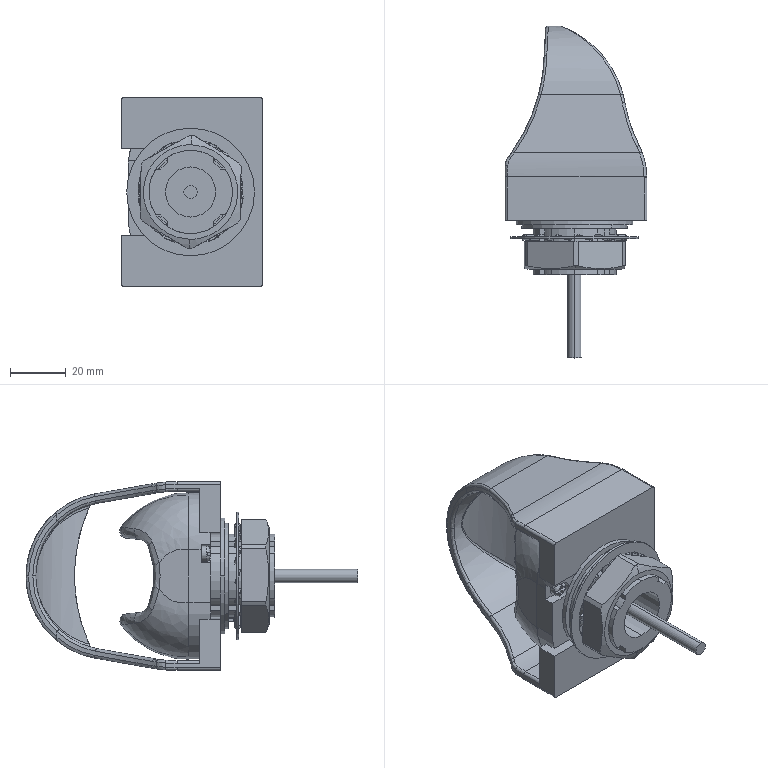Part | SolidWorks | features RefAxis 3 | 6 solids | 600 faces | box 51 x 119.5 x 68 mm | volume 99680 mm3 | cylinder 240 | spline 181 | plane 179 | commonest cylinder face diameters 38 x45 11.374 x28 30.5 x28 2 x20 12.913 x14 12.974 x14